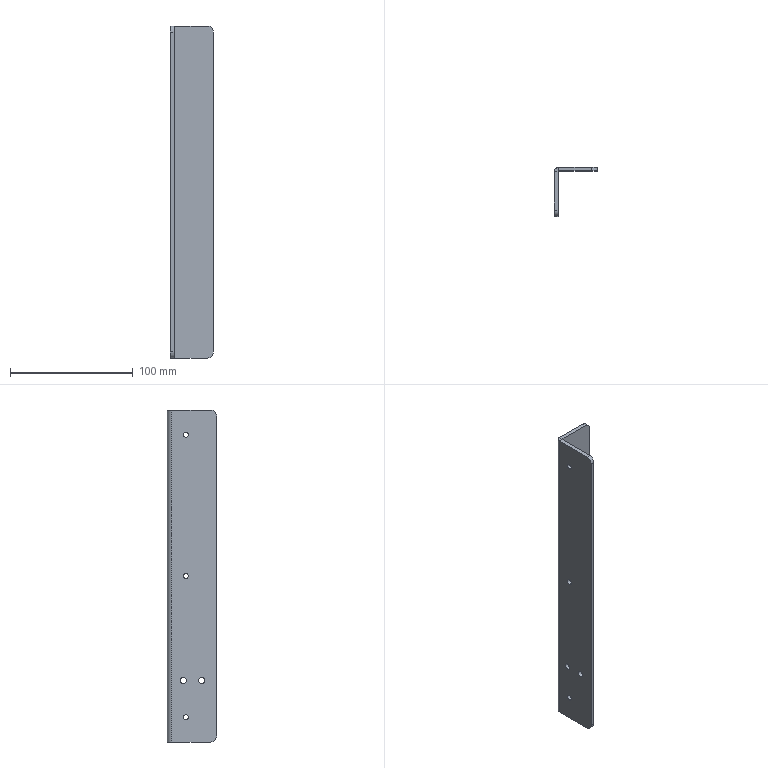Part | SolidWorks | features HoleWzd 2, Fillet 1, FlatPattern 1, SMBaseFlange 1, SheetMetal 1 | 1 solid | 28 faces | box 35 x 40 x 270 mm | volume 57353 mm3 | cylinder 16 | plane 12 | commonest cylinder face diameters 4.2 x6 5 x4 10 x4 0.8 x1 6.8 x1
STEP:
#1=CARTESIAN_POINT('',(-32.,-13.,-82.5));
#2=VERTEX_POINT('',#1);
#3=CARTESIAN_POINT('',(-32.,-13.,-87.5));
#4=VERTEX_POINT('',#3);
#5=CARTESIAN_POINT('',(-32.,-13.,-85.));
#6=DIRECTION('',(1.,0.,0.));
#7=DIRECTION('',(0.,1.,0.));
#8=AXIS2_PLACEMENT_3D('',#5,#6,#7);
#9=CIRCLE('',#8,2.5);
#10=EDGE_CURVE('',#2,#4,#9,.T.);
#11=ORIENTED_EDGE('',*,*,#10,.T.);
#12=CARTESIAN_POINT('',(-35.,-13.,-87.5));
#13=VERTEX_POINT('',#12);
#14=CARTESIAN_POINT('',(-35.,-13.,-87.5));
#15=DIRECTION('',(-1.,0.,0.));
#16=VECTOR('',#15,1000.);
#17=LINE('',#14,#16);
#18=EDGE_CURVE('',#4,#13,#17,.T.);
#19=ORIENTED_EDGE('',*,*,#18,.T.);
#20=CARTESIAN_POINT('',(-35.,-13.,-82.5));
#21=VERTEX_POINT('',#20);
#22=CARTESIAN_POINT('',(-35.,-13.,-85.));
#23=DIRECTION('',(-1.,0.,0.));
#24=DIRECTION('',(0.,0.,1.));
#25=AXIS2_PLACEMENT_3D('',#22,#23,#24);
#26=CIRCLE('',#25,2.5);
#27=EDGE_CURVE('',#13,#21,#26,.T.);
#28=ORIENTED_EDGE('',*,*,#27,.T.);
#29=CARTESIAN_POINT('',(-35.,-13.,-82.5));
#30=DIRECTION('',(-1.,0.,0.));
#31=VECTOR('',#30,1000.);
#32=LINE('',#29,#31);
#33=EDGE_CURVE('',#2,#21,#32,.T.);
#34=ORIENTED_EDGE('',*,*,#33,.F.);
#35=EDGE_LOOP('',(#11,#19,#28,#34));
#36=FACE_OUTER_BOUND('',#35,.T.);
#37=CARTESIAN_POINT('',(-35.,-13.,-85.));
#38=DIRECTION('',(-1.,0.,0.));
#39=DIRECTION('',(0.,0.,1.));
#40=AXIS2_PLACEMENT_3D('',#37,#38,#39);
#41=CYLINDRICAL_SURFACE('',#40,2.5);
#42=ADVANCED_FACE('',(#36),#41,.F.);
#43=CARTESIAN_POINT('',(-32.,-28.,-82.5));
#44=VERTEX_POINT('',#43);
#45=CARTESIAN_POINT('',(-32.,-28.,-87.5));
#46=VERTEX_POINT('',#45);
#47=CARTESIAN_POINT('',(-32.,-28.,-85.));
#48=DIRECTION('',(1.,0.,0.));
#49=DIRECTION('',(0.,1.,0.));
#50=AXIS2_PLACEMENT_3D('',#47,#48,#49);
#51=CIRCLE('',#50,2.5);
#52=EDGE_CURVE('',#44,#46,#51,.T.);
#53=ORIENTED_EDGE('',*,*,#52,.T.);
#54=CARTESIAN_POINT('',(-35.,-28.,-87.5));
#55=VERTEX_POINT('',#54);
#56=CARTESIAN_POINT('',(-35.,-28.,-87.5));
#57=DIRECTION('',(-1.,0.,0.));
#58=VECTOR('',#57,1000.);
#59=LINE('',#56,#58);
#60=EDGE_CURVE('',#46,#55,#59,.T.);
#61=ORIENTED_EDGE('',*,*,#60,.T.);
#62=CARTESIAN_POINT('',(-35.,-28.,-82.5));
#63=VERTEX_POINT('',#62);
#64=CARTESIAN_POINT('',(-35.,-28.,-85.));
#65=DIRECTION('',(-1.,0.,0.));
#66=DIRECTION('',(0.,0.,1.));
#67=AXIS2_PLACEMENT_3D('',#64,#65,#66);
#68=CIRCLE('',#67,2.5);
#69=EDGE_CURVE('',#55,#63,#68,.T.);
#70=ORIENTED_EDGE('',*,*,#69,.T.);
#71=CARTESIAN_POINT('',(-35.,-28.,-82.5));
#72=DIRECTION('',(-1.,0.,0.));
#73=VECTOR('',#72,1000.);
#74=LINE('',#71,#73);
#75=EDGE_CURVE('',#44,#63,#74,.T.);
#76=ORIENTED_EDGE('',*,*,#75,.F.);
#77=EDGE_LOOP('',(#53,#61,#70,#76));
#78=FACE_OUTER_BOUND('',#77,.T.);
#79=CARTESIAN_POINT('',(-35.,-28.,-85.));
#80=DIRECTION('',(-1.,0.,0.));
#81=DIRECTION('',(0.,0.,1.));
#82=AXIS2_PLACEMENT_3D('',#79,#80,#81);
#83=CYLINDRICAL_SURFACE('',#82,2.5);
#84=ADVANCED_FACE('',(#78),#83,.F.);
#85=CARTESIAN_POINT('',(-35.,-15.,117.1));
#86=VERTEX_POINT('',#85);
#87=CARTESIAN_POINT('',(-35.,-15.,112.9));
#88=VERTEX_POINT('',#87);
#89=CARTESIAN_POINT('',(-35.,-15.,115.));
#90=DIRECTION('',(1.,0.,0.));
#91=DIRECTION('',(0.,1.,0.));
#92=AXIS2_PLACEMENT_3D('',#89,#90,#91);
#93=CIRCLE('',#92,2.1);
#94=EDGE_CURVE('',#86,#88,#93,.T.);
#95=ORIENTED_EDGE('',*,*,#94,.F.);
#96=CARTESIAN_POINT('',(-32.,-15.,117.1));
#97=VERTEX_POINT('',#96);
#98=CARTESIAN_POINT('',(-32.,-15.,117.1));
#99=DIRECTION('',(1.,0.,0.));
#100=VECTOR('',#99,1000.);
#101=LINE('',#98,#100);
#102=EDGE_CURVE('',#86,#97,#101,.T.);
#103=ORIENTED_EDGE('',*,*,#102,.T.);
#104=CARTESIAN_POINT('',(-32.,-15.,112.9));
#105=VERTEX_POINT('',#104);
#106=CARTESIAN_POINT('',(-32.,-15.,115.));
#107=DIRECTION('',(1.,0.,0.));
#108=DIRECTION('',(0.,0.,-1.));
#109=AXIS2_PLACEMENT_3D('',#106,#107,#108);
#110=CIRCLE('',#109,2.1);
#111=EDGE_CURVE('',#97,#105,#110,.T.);
#112=ORIENTED_EDGE('',*,*,#111,.T.);
#113=CARTESIAN_POINT('',(-32.,-15.,112.9));
#114=DIRECTION('',(1.,0.,0.));
#115=VECTOR('',#114,1000.);
#116=LINE('',#113,#115);
#117=EDGE_CURVE('',#88,#105,#116,.T.);
#118=ORIENTED_EDGE('',*,*,#117,.F.);
#119=EDGE_LOOP('',(#95,#103,#112,#118));
#120=FACE_OUTER_BOUND('',#119,.T.);
#121=CARTESIAN_POINT('',(-32.,-15.,115.));
#122=DIRECTION('',(1.,0.,0.));
#123=DIRECTION('',(0.,0.,-1.));
#124=AXIS2_PLACEMENT_3D('',#121,#122,#123);
#125=CYLINDRICAL_SURFACE('',#124,2.1);
#126=ADVANCED_FACE('',(#120),#125,.F.);
#127=CARTESIAN_POINT('',(-35.,-15.,-112.9));
#128=VERTEX_POINT('',#127);
#129=CARTESIAN_POINT('',(-35.,-15.,-117.1));
#130=VERTEX_POINT('',#129);
#131=CARTESIAN_POINT('',(-35.,-15.,-115.));
#132=DIRECTION('',(1.,0.,0.));
#133=DIRECTION('',(0.,1.,0.));
#134=AXIS2_PLACEMENT_3D('',#131,#132,#133);
#135=CIRCLE('',#134,2.1);
#136=EDGE_CURVE('',#128,#130,#135,.T.);
#137=ORIENTED_EDGE('',*,*,#136,.F.);
#138=CARTESIAN_POINT('',(-32.,-15.,-112.9));
#139=VERTEX_POINT('',#138);
#140=CARTESIAN_POINT('',(-32.,-15.,-112.9));
#141=DIRECTION('',(1.,0.,0.));
#142=VECTOR('',#141,1000.);
#143=LINE('',#140,#142);
#144=EDGE_CURVE('',#128,#139,#143,.T.);
#145=ORIENTED_EDGE('',*,*,#144,.T.);
#146=CARTESIAN_POINT('',(-32.,-15.,-117.1));
#147=VERTEX_POINT('',#146);
#148=CARTESIAN_POINT('',(-32.,-15.,-115.));
#149=DIRECTION('',(1.,0.,0.));
#150=DIRECTION('',(0.,0.,-1.));
#151=AXIS2_PLACEMENT_3D('',#148,#149,#150);
#152=CIRCLE('',#151,2.1);
#153=EDGE_CURVE('',#139,#147,#152,.T.);
#154=ORIENTED_EDGE('',*,*,#153,.T.);
#155=CARTESIAN_POINT('',(-32.,-15.,-117.1));
#156=DIRECTION('',(1.,0.,0.));
#157=VECTOR('',#156,1000.);
#158=LINE('',#155,#157);
#159=EDGE_CURVE('',#130,#147,#158,.T.);
#160=ORIENTED_EDGE('',*,*,#159,.F.);
#161=EDGE_LOOP('',(#137,#145,#154,#160));
#162=FACE_OUTER_BOUND('',#161,.T.);
#163=CARTESIAN_POINT('',(-32.,-15.,-115.));
#164=DIRECTION('',(1.,0.,0.));
#165=DIRECTION('',(0.,0.,-1.));
#166=AXIS2_PLACEMENT_3D('',#163,#164,#165);
#167=CYLINDRICAL_SURFACE('',#166,2.1);
#168=ADVANCED_FACE('',(#162),#167,.F.);
#169=CARTESIAN_POINT('',(-35.,-15.,2.1));
#170=VERTEX_POINT('',#169);
#171=CARTESIAN_POINT('',(-35.,-15.,-2.1));
#172=VERTEX_POINT('',#171);
#173=CARTESIAN_POINT('',(-35.,-15.,0.));
#174=DIRECTION('',(1.,0.,0.));
#175=DIRECTION('',(0.,1.,0.));
#176=AXIS2_PLACEMENT_3D('',#173,#174,#175);
#177=CIRCLE('',#176,2.1);
#178=EDGE_CURVE('',#170,#172,#177,.T.);
#179=ORIENTED_EDGE('',*,*,#178,.F.);
#180=CARTESIAN_POINT('',(-32.,-15.,2.1));
#181=VERTEX_POINT('',#180);
#182=CARTESIAN_POINT('',(-32.,-15.,2.1));
#183=DIRECTION('',(1.,0.,0.));
#184=VECTOR('',#183,1000.);
#185=LINE('',#182,#184);
#186=EDGE_CURVE('',#170,#181,#185,.T.);
#187=ORIENTED_EDGE('',*,*,#186,.T.);
#188=CARTESIAN_POINT('',(-32.,-15.,-2.1));
#189=VERTEX_POINT('',#188);
#190=CARTESIAN_POINT('',(-32.,-15.,0.));
#191=DIRECTION('',(1.,0.,0.));
#192=DIRECTION('',(0.,0.,-1.));
#193=AXIS2_PLACEMENT_3D('',#190,#191,#192);
#194=CIRCLE('',#193,2.1);
#195=EDGE_CURVE('',#181,#189,#194,.T.);
#196=ORIENTED_EDGE('',*,*,#195,.T.);
#197=CARTESIAN_POINT('',(-32.,-15.,-2.1));
#198=DIRECTION('',(1.,0.,0.));
#199=VECTOR('',#198,1000.);
#200=LINE('',#197,#199);
#201=EDGE_CURVE('',#172,#189,#200,.T.);
#202=ORIENTED_EDGE('',*,*,#201,.F.);
#203=EDGE_LOOP('',(#179,#187,#196,#202));
#204=FACE_OUTER_BOUND('',#203,.T.);
#205=CARTESIAN_POINT('',(-32.,-15.,0.));
#206=DIRECTION('',(1.,0.,0.));
#207=DIRECTION('',(0.,0.,-1.));
#208=AXIS2_PLACEMENT_3D('',#205,#206,#207);
#209=CYLINDRICAL_SURFACE('',#208,2.1);
#210=ADVANCED_FACE('',(#204),#209,.F.);
#211=CARTESIAN_POINT('',(-31.6,0.,135.));
#212=VERTEX_POINT('',#211);
#213=CARTESIAN_POINT('',(-31.6,-3.,135.));
#214=VERTEX_POINT('',#213);
#215=CARTESIAN_POINT('',(-31.6,0.,135.));
#216=DIRECTION('',(0.,-1.,0.));
#217=VECTOR('',#216,1000.);
#218=LINE('',#215,#217);
#219=EDGE_CURVE('',#212,#214,#218,.T.);
#220=ORIENTED_EDGE('',*,*,#219,.F.);
#221=CARTESIAN_POINT('',(-35.,-3.4,135.));
#222=VERTEX_POINT('',#221);
#223=CARTESIAN_POINT('',(-31.6,-3.4,135.));
#224=DIRECTION('',(0.,0.,1.));
#225=DIRECTION('',(-1.,0.,0.));
#226=AXIS2_PLACEMENT_3D('',#223,#224,#225);
#227=CIRCLE('',#226,3.4);
#228=EDGE_CURVE('',#212,#222,#227,.T.);
#229=ORIENTED_EDGE('',*,*,#228,.T.);
#230=CARTESIAN_POINT('',(-32.,-3.4,135.));
#231=VERTEX_POINT('',#230);
#232=CARTESIAN_POINT('',(-32.,-3.4,135.));
#233=DIRECTION('',(-1.,0.,0.));
#234=VECTOR('',#233,1000.);
#235=LINE('',#232,#234);
#236=EDGE_CURVE('',#231,#222,#235,.T.);
#237=ORIENTED_EDGE('',*,*,#236,.F.);
#238=CARTESIAN_POINT('',(-31.6,-3.4,135.));
#239=DIRECTION('',(0.,0.,1.));
#240=DIRECTION('',(1.,0.,0.));
#241=AXIS2_PLACEMENT_3D('',#238,#239,#240);
#242=CIRCLE('',#241,0.4);
#243=EDGE_CURVE('',#214,#231,#242,.T.);
#244=ORIENTED_EDGE('',*,*,#243,.F.);
#245=EDGE_LOOP('',(#220,#229,#237,#244));
#246=FACE_OUTER_BOUND('',#245,.T.);
#247=CARTESIAN_POINT('',(-31.6,0.,135.));
#248=DIRECTION('',(0.,0.,1.));
#249=DIRECTION('',(1.,0.,0.));
#250=AXIS2_PLACEMENT_3D('',#247,#248,#249);
#251=PLANE('',#250);
#252=ADVANCED_FACE('',(#246),#251,.T.);
#253=CARTESIAN_POINT('',(-5.,-3.,135.));
#254=VERTEX_POINT('',#253);
#255=CARTESIAN_POINT('',(0.,-3.,135.));
#256=DIRECTION('',(-1.,0.,0.));
#257=VECTOR('',#256,1000.);
#258=LINE('',#255,#257);
#259=EDGE_CURVE('',#254,#214,#258,.T.);
#260=ORIENTED_EDGE('',*,*,#259,.F.);
#261=CARTESIAN_POINT('',(-5.,0.,135.));
#262=VERTEX_POINT('',#261);
#263=CARTESIAN_POINT('',(-5.,-3.4,135.));
#264=DIRECTION('',(0.,1.,0.));
#265=VECTOR('',#264,1000.);
#266=LINE('',#263,#265);
#267=EDGE_CURVE('',#254,#262,#266,.T.);
#268=ORIENTED_EDGE('',*,*,#267,.T.);
#269=CARTESIAN_POINT('',(0.,0.,135.));
#270=DIRECTION('',(-1.,0.,0.));
#271=VECTOR('',#270,1000.);
#272=LINE('',#269,#271);
#273=EDGE_CURVE('',#262,#212,#272,.T.);
#274=ORIENTED_EDGE('',*,*,#273,.T.);
#275=ORIENTED_EDGE('',*,*,#219,.T.);
#276=EDGE_LOOP('',(#260,#268,#274,#275));
#277=FACE_OUTER_BOUND('',#276,.T.);
#278=CARTESIAN_POINT('',(-32.,-3.4,135.));
#279=DIRECTION('',(0.,0.,1.));
#280=DIRECTION('',(1.,0.,0.));
#281=AXIS2_PLACEMENT_3D('',#278,#279,#280);
#282=PLANE('',#281);
#283=ADVANCED_FACE('',(#277),#282,.T.);
#284=CARTESIAN_POINT('',(-35.,-3.4,-135.));
#285=VERTEX_POINT('',#284);
#286=CARTESIAN_POINT('',(-32.,-3.4,-135.));
#287=VERTEX_POINT('',#286);
#288=CARTESIAN_POINT('',(-35.,-3.4,-135.));
#289=DIRECTION('',(1.,0.,0.));
#290=VECTOR('',#289,1000.);
#291=LINE('',#288,#290);
#292=EDGE_CURVE('',#285,#287,#291,.T.);
#293=ORIENTED_EDGE('',*,*,#292,.F.);
#294=CARTESIAN_POINT('',(-31.6,0.,-135.));
#295=VERTEX_POINT('',#294);
#296=CARTESIAN_POINT('',(-31.6,-3.4,-135.));
#297=DIRECTION('',(0.,0.,1.));
#298=DIRECTION('',(-1.,0.,0.));
#299=AXIS2_PLACEMENT_3D('',#296,#297,#298);
#300=CIRCLE('',#299,3.4);
#301=EDGE_CURVE('',#295,#285,#300,.T.);
#302=ORIENTED_EDGE('',*,*,#301,.F.);
#303=CARTESIAN_POINT('',(-31.6,-3.,-135.));
#304=VERTEX_POINT('',#303);
#305=CARTESIAN_POINT('',(-31.6,-3.,-135.));
#306=DIRECTION('',(0.,1.,0.));
#307=VECTOR('',#306,1000.);
#308=LINE('',#305,#307);
#309=EDGE_CURVE('',#304,#295,#308,.T.);
#310=ORIENTED_EDGE('',*,*,#309,.F.);
#311=CARTESIAN_POINT('',(-31.6,-3.4,-135.));
#312=DIRECTION('',(0.,0.,1.));
#313=DIRECTION('',(1.,0.,0.));
#314=AXIS2_PLACEMENT_3D('',#311,#312,#313);
#315=CIRCLE('',#314,0.4);
#316=EDGE_CURVE('',#304,#287,#315,.T.);
#317=ORIENTED_EDGE('',*,*,#316,.T.);
#318=EDGE_LOOP('',(#293,#302,#310,#317));
#319=FACE_OUTER_BOUND('',#318,.T.);
#320=CARTESIAN_POINT('',(-35.,-3.4,-135.));
#321=DIRECTION('',(0.,0.,-1.));
#322=DIRECTION('',(-1.,0.,0.));
#323=AXIS2_PLACEMENT_3D('',#320,#321,#322);
#324=PLANE('',#323);
#325=ADVANCED_FACE('',(#319),#324,.T.);
#326=CARTESIAN_POINT('',(-32.,-35.,-135.));
#327=VERTEX_POINT('',#326);
#328=CARTESIAN_POINT('',(-32.,0.,-135.));
#329=DIRECTION('',(0.,-1.,0.));
#330=VECTOR('',#329,1000.);
#331=LINE('',#328,#330);
#332=EDGE_CURVE('',#287,#327,#331,.T.);
#333=ORIENTED_EDGE('',*,*,#332,.T.);
#334=CARTESIAN_POINT('',(-35.,-35.,-135.));
#335=VERTEX_POINT('',#334);
#336=CARTESIAN_POINT('',(-31.6,-35.,-135.));
#337=DIRECTION('',(-1.,0.,0.));
#338=VECTOR('',#337,1000.);
#339=LINE('',#336,#338);
#340=EDGE_CURVE('',#327,#335,#339,.T.);
#341=ORIENTED_EDGE('',*,*,#340,.T.);
#342=CARTESIAN_POINT('',(-35.,0.,-135.));
#343=DIRECTION('',(0.,-1.,0.));
#344=VECTOR('',#343,1000.);
#345=LINE('',#342,#344);
#346=EDGE_CURVE('',#285,#335,#345,.T.);
#347=ORIENTED_EDGE('',*,*,#346,.F.);
#348=ORIENTED_EDGE('',*,*,#292,.T.);
#349=EDGE_LOOP('',(#333,#341,#347,#348));
#350=FACE_OUTER_BOUND('',#349,.T.);
#351=CARTESIAN_POINT('',(-31.6,-3.,-135.));
#352=DIRECTION('',(0.,0.,-1.));
#353=DIRECTION('',(-1.,0.,0.));
#354=AXIS2_PLACEMENT_3D('',#351,#352,#353);
#355=PLANE('',#354);
#356=ADVANCED_FACE('',(#350),#355,.T.);
#357=CARTESIAN_POINT('',(-35.,-13.,-85.));
#358=DIRECTION('',(-1.,0.,0.));
#359=DIRECTION('',(0.,0.,1.));
#360=AXIS2_PLACEMENT_3D('',#357,#358,#359);
#361=CIRCLE('',#360,2.5);
#362=EDGE_CURVE('',#21,#13,#361,.T.);
#363=ORIENTED_EDGE('',*,*,#362,.F.);
#364=ORIENTED_EDGE('',*,*,#27,.F.);
#365=EDGE_LOOP('',(#363,#364));
#366=FACE_BOUND('',#365,.T.);
#367=CARTESIAN_POINT('',(-35.,-28.,-85.));
#368=DIRECTION('',(-1.,0.,0.));
#369=DIRECTION('',(0.,0.,1.));
#370=AXIS2_PLACEMENT_3D('',#367,#368,#369);
#371=CIRCLE('',#370,2.5);
#372=EDGE_CURVE('',#63,#55,#371,.T.);
#373=ORIENTED_EDGE('',*,*,#372,.F.);
#374=ORIENTED_EDGE('',*,*,#69,.F.);
#375=EDGE_LOOP('',(#373,#374));
#376=FACE_BOUND('',#375,.T.);
#377=CARTESIAN_POINT('',(-35.,-15.,115.));
#378=DIRECTION('',(1.,0.,0.));
#379=DIRECTION('',(0.,1.,0.));
#380=AXIS2_PLACEMENT_3D('',#377,#378,#379);
#381=CIRCLE('',#380,2.1);
#382=EDGE_CURVE('',#88,#86,#381,.T.);
#383=ORIENTED_EDGE('',*,*,#382,.T.);
#384=ORIENTED_EDGE('',*,*,#94,.T.);
#385=EDGE_LOOP('',(#383,#384));
#386=FACE_BOUND('',#385,.T.);
#387=CARTESIAN_POINT('',(-35.,-15.,-115.));
#388=DIRECTION('',(1.,0.,0.));
#389=DIRECTION('',(0.,1.,0.));
#390=AXIS2_PLACEMENT_3D('',#387,#388,#389);
#391=CIRCLE('',#390,2.1);
#392=EDGE_CURVE('',#130,#128,#391,.T.);
#393=ORIENTED_EDGE('',*,*,#392,.T.);
#394=ORIENTED_EDGE('',*,*,#136,.T.);
#395=EDGE_LOOP('',(#393,#394));
#396=FACE_BOUND('',#395,.T.);
#397=CARTESIAN_POINT('',(-35.,-15.,0.));
#398=DIRECTION('',(1.,0.,0.));
#399=DIRECTION('',(0.,1.,0.));
#400=AXIS2_PLACEMENT_3D('',#397,#398,#399);
#401=CIRCLE('',#400,2.1);
#402=EDGE_CURVE('',#172,#170,#401,.T.);
#403=ORIENTED_EDGE('',*,*,#402,.T.);
#404=ORIENTED_EDGE('',*,*,#178,.T.);
#405=EDGE_LOOP('',(#403,#404));
#406=FACE_BOUND('',#405,.T.);
#407=ORIENTED_EDGE('',*,*,#346,.T.);
#408=CARTESIAN_POINT('',(-35.,-40.,-130.));
#409=VERTEX_POINT('',#408);
#410=CARTESIAN_POINT('',(-35.,-35.,-130.));
#411=DIRECTION('',(-1.,0.,0.));
#412=DIRECTION('',(0.,1.,0.));
#413=AXIS2_PLACEMENT_3D('',#410,#411,#412);
#414=CIRCLE('',#413,5.);
#415=EDGE_CURVE('',#335,#409,#414,.T.);
#416=ORIENTED_EDGE('',*,*,#415,.T.);
#417=CARTESIAN_POINT('',(-35.,-40.,130.));
#418=VERTEX_POINT('',#417);
#419=CARTESIAN_POINT('',(-35.,-40.,135.));
#420=DIRECTION('',(0.,0.,-1.));
#421=VECTOR('',#420,1000.);
#422=LINE('',#419,#421);
#423=EDGE_CURVE('',#418,#409,#422,.T.);
#424=ORIENTED_EDGE('',*,*,#423,.F.);
#425=CARTESIAN_POINT('',(-35.,-35.,135.));
#426=VERTEX_POINT('',#425);
#427=CARTESIAN_POINT('',(-35.,-35.,130.));
#428=DIRECTION('',(-1.,0.,0.));
#429=DIRECTION('',(0.,1.,0.));
#430=AXIS2_PLACEMENT_3D('',#427,#428,#429);
#431=CIRCLE('',#430,5.);
#432=EDGE_CURVE('',#418,#426,#431,.T.);
#433=ORIENTED_EDGE('',*,*,#432,.T.);
#434=CARTESIAN_POINT('',(-35.,0.,135.));
#435=DIRECTION('',(0.,-1.,0.));
#436=VECTOR('',#435,1000.);
#437=LINE('',#434,#436);
#438=EDGE_CURVE('',#222,#426,#437,.T.);
#439=ORIENTED_EDGE('',*,*,#438,.F.);
#440=CARTESIAN_POINT('',(-35.,-3.4,135.));
#441=DIRECTION('',(0.,0.,-1.));
#442=VECTOR('',#441,1000.);
#443=LINE('',#440,#442);
#444=EDGE_CURVE('',#222,#285,#443,.T.);
#445=ORIENTED_EDGE('',*,*,#444,.T.);
#446=EDGE_LOOP('',(#407,#416,#424,#433,#439,#445));
#447=FACE_OUTER_BOUND('',#446,.T.);
#448=CARTESIAN_POINT('',(-35.,0.,135.));
#449=DIRECTION('',(1.,0.,0.));
#450=DIRECTION('',(0.,1.,0.));
#451=AXIS2_PLACEMENT_3D('',#448,#449,#450);
#452=PLANE('',#451);
#453=ADVANCED_FACE('',(#366,#376,#386,#396,#406,#447),#452,.F.);
#454=ORIENTED_EDGE('',*,*,#423,.T.);
#455=CARTESIAN_POINT('',(-32.,-40.,-130.));
#456=VERTEX_POINT('',#455);
#457=CARTESIAN_POINT('',(-32.,-40.,-130.));
#458=DIRECTION('',(1.,0.,0.));
#459=VECTOR('',#458,1000.);
#460=LINE('',#457,#459);
#461=EDGE_CURVE('',#409,#456,#460,.T.);
#462=ORIENTED_EDGE('',*,*,#461,.T.);
#463=CARTESIAN_POINT('',(-32.,-40.,130.));
#464=VERTEX_POINT('',#463);
#465=CARTESIAN_POINT('',(-32.,-40.,135.));
#466=DIRECTION('',(0.,0.,-1.));
#467=VECTOR('',#466,1000.);
#468=LINE('',#465,#467);
#469=EDGE_CURVE('',#464,#456,#468,.T.);
#470=ORIENTED_EDGE('',*,*,#469,.F.);
#471=CARTESIAN_POINT('',(-32.,-40.,130.));
#472=DIRECTION('',(-1.,0.,0.));
#473=VECTOR('',#472,1000.);
#474=LINE('',#471,#473);
#475=EDGE_CURVE('',#464,#418,#474,.T.);
#476=ORIENTED_EDGE('',*,*,#475,.T.);
#477=EDGE_LOOP('',(#454,#462,#470,#476));
#478=FACE_OUTER_BOUND('',#477,.T.);
#479=CARTESIAN_POINT('',(-32.,-40.,135.));
#480=DIRECTION('',(0.,-1.,0.));
#481=DIRECTION('',(0.,0.,-1.));
#482=AXIS2_PLACEMENT_3D('',#479,#480,#481);
#483=PLANE('',#482);
#484=ADVANCED_FACE('',(#478),#483,.T.);
#485=ORIENTED_EDGE('',*,*,#10,.F.);
#486=CARTESIAN_POINT('',(-32.,-13.,-85.));
#487=DIRECTION('',(1.,0.,0.));
#488=DIRECTION('',(0.,1.,0.));
#489=AXIS2_PLACEMENT_3D('',#486,#487,#488);
#490=CIRCLE('',#489,2.5);
#491=EDGE_CURVE('',#4,#2,#490,.T.);
#492=ORIENTED_EDGE('',*,*,#491,.F.);
#493=EDGE_LOOP('',(#485,#492));
#494=FACE_BOUND('',#493,.T.);
#495=ORIENTED_EDGE('',*,*,#52,.F.);
#496=CARTESIAN_POINT('',(-32.,-28.,-85.));
#497=DIRECTION('',(1.,0.,0.));
#498=DIRECTION('',(0.,1.,0.));
#499=AXIS2_PLACEMENT_3D('',#496,#497,#498);
#500=CIRCLE('',#499,2.5);
#501=EDGE_CURVE('',#46,#44,#500,.T.);
#502=ORIENTED_EDGE('',*,*,#501,.F.);
#503=EDGE_LOOP('',(#495,#502));
#504=FACE_BOUND('',#503,.T.);
#505=CARTESIAN_POINT('',(-32.,-15.,115.));
#506=DIRECTION('',(1.,0.,0.));
#507=DIRECTION('',(0.,0.,-1.));
#508=AXIS2_PLACEMENT_3D('',#505,#506,#507);
#509=CIRCLE('',#508,2.1);
#510=EDGE_CURVE('',#105,#97,#509,.T.);
#511=ORIENTED_EDGE('',*,*,#510,.F.);
#512=ORIENTED_EDGE('',*,*,#111,.F.);
#513=EDGE_LOOP('',(#511,#512));
#514=FACE_BOUND('',#513,.T.);
#515=CARTESIAN_POINT('',(-32.,-15.,-115.));
#516=DIRECTION('',(1.,0.,0.));
#517=DIRECTION('',(0.,0.,-1.));
#518=AXIS2_PLACEMENT_3D('',#515,#516,#517);
#519=CIRCLE('',#518,2.1);
#520=EDGE_CURVE('',#147,#139,#519,.T.);
#521=ORIENTED_EDGE('',*,*,#520,.F.);
#522=ORIENTED_EDGE('',*,*,#153,.F.);
#523=EDGE_LOOP('',(#521,#522));
#524=FACE_BOUND('',#523,.T.);
#525=CARTESIAN_POINT('',(-32.,-15.,0.));
#526=DIRECTION('',(1.,0.,0.));
#527=DIRECTION('',(0.,0.,-1.));
#528=AXIS2_PLACEMENT_3D('',#525,#526,#527);
#529=CIRCLE('',#528,2.1);
#530=EDGE_CURVE('',#189,#181,#529,.T.);
#531=ORIENTED_EDGE('',*,*,#530,.F.);
#532=ORIENTED_EDGE('',*,*,#195,.F.);
#533=EDGE_LOOP('',(#531,#532));
#534=FACE_BOUND('',#533,.T.);
#535=ORIENTED_EDGE('',*,*,#469,.T.);
#536=CARTESIAN_POINT('',(-32.,-35.,-130.));
#537=DIRECTION('',(1.,0.,0.));
#538=DIRECTION('',(0.,1.,0.));
#539=AXIS2_PLACEMENT_3D('',#536,#537,#538);
#540=CIRCLE('',#539,5.);
#541=EDGE_CURVE('',#456,#327,#540,.T.);
#542=ORIENTED_EDGE('',*,*,#541,.T.);
#543=ORIENTED_EDGE('',*,*,#332,.F.);
#544=CARTESIAN_POINT('',(-32.,-3.4,135.));
#545=DIRECTION('',(0.,0.,-1.));
#546=VECTOR('',#545,1000.);
#547=LINE('',#544,#546);
#548=EDGE_CURVE('',#231,#287,#547,.T.);
#549=ORIENTED_EDGE('',*,*,#548,.F.);
#550=CARTESIAN_POINT('',(-32.,-35.,135.));
#551=VERTEX_POINT('',#550);
#552=CARTESIAN_POINT('',(-32.,0.,135.));
#553=DIRECTION('',(0.,-1.,0.));
#554=VECTOR('',#553,1000.);
#555=LINE('',#552,#554);
#556=EDGE_CURVE('',#231,#551,#555,.T.);
#557=ORIENTED_EDGE('',*,*,#556,.T.);
#558=CARTESIAN_POINT('',(-32.,-35.,130.));
#559=DIRECTION('',(1.,0.,0.));
#560=DIRECTION('',(0.,1.,0.));
#561=AXIS2_PLACEMENT_3D('',#558,#559,#560);
#562=CIRCLE('',#561,5.);
#563=EDGE_CURVE('',#551,#464,#562,.T.);
#564=ORIENTED_EDGE('',*,*,#563,.T.);
#565=EDGE_LOOP('',(#535,#542,#543,#549,#557,#564));
#566=FACE_OUTER_BOUND('',#565,.T.);
#567=CARTESIAN_POINT('',(-32.,0.,135.));
#568=DIRECTION('',(1.,0.,0.));
#569=DIRECTION('',(0.,1.,0.));
#570=AXIS2_PLACEMENT_3D('',#567,#568,#569);
#571=PLANE('',#570);
#572=ADVANCED_FACE('',(#494,#504,#514,#524,#534,#566),#571,.T.);
#573=ORIENTED_EDGE('',*,*,#316,.F.);
#574=CARTESIAN_POINT('',(-31.6,-3.,135.));
#575=DIRECTION('',(0.,0.,-1.));
#576=VECTOR('',#575,1000.);
#577=LINE('',#574,#576);
#578=EDGE_CURVE('',#214,#304,#577,.T.);
#579=ORIENTED_EDGE('',*,*,#578,.F.);
#580=ORIENTED_EDGE('',*,*,#243,.T.);
#581=ORIENTED_EDGE('',*,*,#548,.T.);
#582=EDGE_LOOP('',(#573,#579,#580,#581));
#583=FACE_OUTER_BOUND('',#582,.T.);
#584=CARTESIAN_POINT('',(-31.6,-3.4,135.));
#585=DIRECTION('',(0.,0.,-1.));
#586=DIRECTION('',(-1.,0.,0.));
#587=AXIS2_PLACEMENT_3D('',#584,#585,#586);
#588=CYLINDRICAL_SURFACE('',#587,0.4);
#589=ADVANCED_FACE('',(#583),#588,.F.);
#590=CARTESIAN_POINT('',(-5.,-3.,-135.));
#591=VERTEX_POINT('',#590);
#592=CARTESIAN_POINT('',(0.,-3.,-135.));
#593=DIRECTION('',(-1.,0.,0.));
#594=VECTOR('',#593,1000.);
#595=LINE('',#592,#594);
#596=EDGE_CURVE('',#591,#304,#595,.T.);
#597=ORIENTED_EDGE('',*,*,#596,.F.);
#598=CARTESIAN_POINT('',(0.,-3.,-130.));
#599=VERTEX_POINT('',#598);
#600=CARTESIAN_POINT('',(-5.,-3.,-130.));
#601=DIRECTION('',(0.,-1.,0.));
#602=DIRECTION('',(0.,0.,-1.));
#603=AXIS2_PLACEMENT_3D('',#600,#601,#602);
#604=CIRCLE('',#603,5.);
#605=EDGE_CURVE('',#591,#599,#604,.T.);
#606=ORIENTED_EDGE('',*,*,#605,.T.);
#607=CARTESIAN_POINT('',(0.,-3.,130.));
#608=VERTEX_POINT('',#607);
#609=CARTESIAN_POINT('',(0.,-3.,135.));
#610=DIRECTION('',(0.,0.,-1.));
#611=VECTOR('',#610,1000.);
#612=LINE('',#609,#611);
#613=EDGE_CURVE('',#608,#599,#612,.T.);
#614=ORIENTED_EDGE('',*,*,#613,.F.);
#615=CARTESIAN_POINT('',(-5.,-3.,130.));
#616=DIRECTION('',(0.,-1.,0.));
#617=DIRECTION('',(0.,0.,-1.));
#618=AXIS2_PLACEMENT_3D('',#615,#616,#617);
#619=CIRCLE('',#618,5.);
#620=EDGE_CURVE('',#608,#254,#619,.T.);
#621=ORIENTED_EDGE('',*,*,#620,.T.);
#622=ORIENTED_EDGE('',*,*,#259,.T.);
#623=ORIENTED_EDGE('',*,*,#578,.T.);
#624=EDGE_LOOP('',(#597,#606,#614,#621,#622,#623));
#625=FACE_OUTER_BOUND('',#624,.T.);
#626=CARTESIAN_POINT('',(0.,-3.,135.));
#627=DIRECTION('',(0.,-1.,0.));
#628=DIRECTION('',(0.,0.,-1.));
#629=AXIS2_PLACEMENT_3D('',#626,#627,#628);
#630=PLANE('',#629);
#631=ADVANCED_FACE('',(#625),#630,.T.);
#632=ORIENTED_EDGE('',*,*,#613,.T.);
#633=CARTESIAN_POINT('',(0.,0.,-130.));
#634=VERTEX_POINT('',#633);
#635=CARTESIAN_POINT('',(0.,0.,-130.));
#636=DIRECTION('',(0.,1.,0.));
#637=VECTOR('',#636,1000.);
#638=LINE('',#635,#637);
#639=EDGE_CURVE('',#599,#634,#638,.T.);
#640=ORIENTED_EDGE('',*,*,#639,.T.);
#641=CARTESIAN_POINT('',(0.,0.,130.));
#642=VERTEX_POINT('',#641);
#643=CARTESIAN_POINT('',(0.,0.,135.));
#644=DIRECTION('',(0.,0.,-1.));
#645=VECTOR('',#644,1000.);
#646=LINE('',#643,#645);
#647=EDGE_CURVE('',#642,#634,#646,.T.);
#648=ORIENTED_EDGE('',*,*,#647,.F.);
#649=CARTESIAN_POINT('',(0.,0.,130.));
#650=DIRECTION('',(0.,-1.,0.));
#651=VECTOR('',#650,1000.);
#652=LINE('',#649,#651);
#653=EDGE_CURVE('',#642,#608,#652,.T.);
#654=ORIENTED_EDGE('',*,*,#653,.T.);
#655=EDGE_LOOP('',(#632,#640,#648,#654));
#656=FACE_OUTER_BOUND('',#655,.T.);
#657=CARTESIAN_POINT('',(0.,0.,135.));
#658=DIRECTION('',(1.,0.,0.));
#659=DIRECTION('',(0.,0.,-1.));
#660=AXIS2_PLACEMENT_3D('',#657,#658,#659);
#661=PLANE('',#660);
#662=ADVANCED_FACE('',(#656),#661,.T.);
#663=ORIENTED_EDGE('',*,*,#647,.T.);
#664=CARTESIAN_POINT('',(-5.,0.,-135.));
#665=VERTEX_POINT('',#664);
#666=CARTESIAN_POINT('',(-5.,0.,-130.));
#667=DIRECTION('',(0.,1.,0.));
#668=DIRECTION('',(0.,0.,-1.));
#669=AXIS2_PLACEMENT_3D('',#666,#667,#668);
#670=CIRCLE('',#669,5.);
#671=EDGE_CURVE('',#634,#665,#670,.T.);
#672=ORIENTED_EDGE('',*,*,#671,.T.);
#673=CARTESIAN_POINT('',(0.,0.,-135.));
#674=DIRECTION('',(-1.,0.,0.));
#675=VECTOR('',#674,1000.);
#676=LINE('',#673,#675);
#677=EDGE_CURVE('',#665,#295,#676,.T.);
#678=ORIENTED_EDGE('',*,*,#677,.T.);
#679=CARTESIAN_POINT('',(-31.6,0.,135.));
#680=DIRECTION('',(0.,0.,-1.));
#681=VECTOR('',#680,1000.);
#682=LINE('',#679,#681);
#683=EDGE_CURVE('',#212,#295,#682,.T.);
#684=ORIENTED_EDGE('',*,*,#683,.F.);
#685=ORIENTED_EDGE('',*,*,#273,.F.);
#686=CARTESIAN_POINT('',(-5.,0.,130.));
#687=DIRECTION('',(0.,1.,0.));
#688=DIRECTION('',(0.,0.,-1.));
#689=AXIS2_PLACEMENT_3D('',#686,#687,#688);
#690=CIRCLE('',#689,5.);
#691=EDGE_CURVE('',#262,#642,#690,.T.);
#692=ORIENTED_EDGE('',*,*,#691,.T.);
#693=EDGE_LOOP('',(#663,#672,#678,#684,#685,#692));
#694=FACE_OUTER_BOUND('',#693,.T.);
#695=CARTESIAN_POINT('',(0.,0.,135.));
#696=DIRECTION('',(0.,-1.,0.));
#697=DIRECTION('',(0.,0.,-1.));
#698=AXIS2_PLACEMENT_3D('',#695,#696,#697);
#699=PLANE('',#698);
#700=ADVANCED_FACE('',(#694),#699,.F.);
#701=ORIENTED_EDGE('',*,*,#301,.T.);
#702=ORIENTED_EDGE('',*,*,#444,.F.);
#703=ORIENTED_EDGE('',*,*,#228,.F.);
#704=ORIENTED_EDGE('',*,*,#683,.T.);
#705=EDGE_LOOP('',(#701,#702,#703,#704));
#706=FACE_OUTER_BOUND('',#705,.T.);
#707=CARTESIAN_POINT('',(-31.6,-3.4,135.));
#708=DIRECTION('',(0.,0.,-1.));
#709=DIRECTION('',(-1.,0.,0.));
#710=AXIS2_PLACEMENT_3D('',#707,#708,#709);
#711=CYLINDRICAL_SURFACE('',#710,3.4);
#712=ADVANCED_FACE('',(#706),#711,.T.);
#713=ORIENTED_EDGE('',*,*,#438,.T.);
#714=CARTESIAN_POINT('',(-31.6,-35.,135.));
#715=DIRECTION('',(1.,0.,0.));
#716=VECTOR('',#715,1000.);
#717=LINE('',#714,#716);
#718=EDGE_CURVE('',#426,#551,#717,.T.);
#719=ORIENTED_EDGE('',*,*,#718,.T.);
#720=ORIENTED_EDGE('',*,*,#556,.F.);
#721=ORIENTED_EDGE('',*,*,#236,.T.);
#722=EDGE_LOOP('',(#713,#719,#720,#721));
#723=FACE_OUTER_BOUND('',#722,.T.);
#724=CARTESIAN_POINT('',(-31.6,-3.4,135.));
#725=DIRECTION('',(0.,0.,1.));
#726=DIRECTION('',(1.,0.,0.));
#727=AXIS2_PLACEMENT_3D('',#724,#725,#726);
#728=PLANE('',#727);
#729=ADVANCED_FACE('',(#723),#728,.T.);
#730=ORIENTED_EDGE('',*,*,#677,.F.);
#731=CARTESIAN_POINT('',(-5.,-3.,-135.));
#732=DIRECTION('',(0.,-1.,0.));
#733=VECTOR('',#732,1000.);
#734=LINE('',#731,#733);
#735=EDGE_CURVE('',#665,#591,#734,.T.);
#736=ORIENTED_EDGE('',*,*,#735,.T.);
#737=ORIENTED_EDGE('',*,*,#596,.T.);
#738=ORIENTED_EDGE('',*,*,#309,.T.);
#739=EDGE_LOOP('',(#730,#736,#737,#738));
#740=FACE_OUTER_BOUND('',#739,.T.);
#741=CARTESIAN_POINT('',(-31.6,-3.4,-135.));
#742=DIRECTION('',(0.,0.,1.));
#743=DIRECTION('',(1.,0.,0.));
#744=AXIS2_PLACEMENT_3D('',#741,#742,#743);
#745=PLANE('',#744);
#746=ADVANCED_FACE('',(#740),#745,.F.);
#747=ORIENTED_EDGE('',*,*,#186,.F.);
#748=ORIENTED_EDGE('',*,*,#402,.F.);
#749=ORIENTED_EDGE('',*,*,#201,.T.);
#750=ORIENTED_EDGE('',*,*,#530,.T.);
#751=EDGE_LOOP('',(#747,#748,#749,#750));
#752=FACE_OUTER_BOUND('',#751,.T.);
#753=CARTESIAN_POINT('',(-32.,-15.,0.));
#754=DIRECTION('',(1.,0.,0.));
#755=DIRECTION('',(0.,0.,-1.));
#756=AXIS2_PLACEMENT_3D('',#753,#754,#755);
#757=CYLINDRICAL_SURFACE('',#756,2.1);
#758=ADVANCED_FACE('',(#752),#757,.F.);
#759=ORIENTED_EDGE('',*,*,#144,.F.);
#760=ORIENTED_EDGE('',*,*,#392,.F.);
#761=ORIENTED_EDGE('',*,*,#159,.T.);
#762=ORIENTED_EDGE('',*,*,#520,.T.);
#763=EDGE_LOOP('',(#759,#760,#761,#762));
#764=FACE_OUTER_BOUND('',#763,.T.);
#765=CARTESIAN_POINT('',(-32.,-15.,-115.));
#766=DIRECTION('',(1.,0.,0.));
#767=DIRECTION('',(0.,0.,-1.));
#768=AXIS2_PLACEMENT_3D('',#765,#766,#767);
#769=CYLINDRICAL_SURFACE('',#768,2.1);
#770=ADVANCED_FACE('',(#764),#769,.F.);
#771=ORIENTED_EDGE('',*,*,#102,.F.);
#772=ORIENTED_EDGE('',*,*,#382,.F.);
#773=ORIENTED_EDGE('',*,*,#117,.T.);
#774=ORIENTED_EDGE('',*,*,#510,.T.);
#775=EDGE_LOOP('',(#771,#772,#773,#774));
#776=FACE_OUTER_BOUND('',#775,.T.);
#777=CARTESIAN_POINT('',(-32.,-15.,115.));
#778=DIRECTION('',(1.,0.,0.));
#779=DIRECTION('',(0.,0.,-1.));
#780=AXIS2_PLACEMENT_3D('',#777,#778,#779);
#781=CYLINDRICAL_SURFACE('',#780,2.1);
#782=ADVANCED_FACE('',(#776),#781,.F.);
#783=ORIENTED_EDGE('',*,*,#541,.F.);
#784=ORIENTED_EDGE('',*,*,#461,.F.);
#785=ORIENTED_EDGE('',*,*,#415,.F.);
#786=ORIENTED_EDGE('',*,*,#340,.F.);
#787=EDGE_LOOP('',(#783,#784,#785,#786));
#788=FACE_OUTER_BOUND('',#787,.T.);
#789=CARTESIAN_POINT('',(-31.6,-35.,-130.));
#790=DIRECTION('',(-1.,0.,0.));
#791=DIRECTION('',(0.,0.,1.));
#792=AXIS2_PLACEMENT_3D('',#789,#790,#791);
#793=CYLINDRICAL_SURFACE('',#792,5.);
#794=ADVANCED_FACE('',(#788),#793,.T.);
#795=ORIENTED_EDGE('',*,*,#671,.F.);
#796=ORIENTED_EDGE('',*,*,#639,.F.);
#797=ORIENTED_EDGE('',*,*,#605,.F.);
#798=ORIENTED_EDGE('',*,*,#735,.F.);
#799=EDGE_LOOP('',(#795,#796,#797,#798));
#800=FACE_OUTER_BOUND('',#799,.T.);
#801=CARTESIAN_POINT('',(-5.,-3.4,-130.));
#802=DIRECTION('',(0.,1.,0.));
#803=DIRECTION('',(0.,0.,1.));
#804=AXIS2_PLACEMENT_3D('',#801,#802,#803);
#805=CYLINDRICAL_SURFACE('',#804,5.);
#806=ADVANCED_FACE('',(#800),#805,.T.);
#807=ORIENTED_EDGE('',*,*,#563,.F.);
#808=ORIENTED_EDGE('',*,*,#718,.F.);
#809=ORIENTED_EDGE('',*,*,#432,.F.);
#810=ORIENTED_EDGE('',*,*,#475,.F.);
#811=EDGE_LOOP('',(#807,#808,#809,#810));
#812=FACE_OUTER_BOUND('',#811,.T.);
#813=CARTESIAN_POINT('',(-32.,-35.,130.));
#814=DIRECTION('',(-1.,0.,0.));
#815=DIRECTION('',(0.,0.,1.));
#816=AXIS2_PLACEMENT_3D('',#813,#814,#815);
#817=CYLINDRICAL_SURFACE('',#816,5.);
#818=ADVANCED_FACE('',(#812),#817,.T.);
#819=ORIENTED_EDGE('',*,*,#691,.F.);
#820=ORIENTED_EDGE('',*,*,#267,.F.);
#821=ORIENTED_EDGE('',*,*,#620,.F.);
#822=ORIENTED_EDGE('',*,*,#653,.F.);
#823=EDGE_LOOP('',(#819,#820,#821,#822));
#824=FACE_OUTER_BOUND('',#823,.T.);
#825=CARTESIAN_POINT('',(-5.,0.,130.));
#826=DIRECTION('',(0.,-1.,0.));
#827=DIRECTION('',(0.,0.,-1.));
#828=AXIS2_PLACEMENT_3D('',#825,#826,#827);
#829=CYLINDRICAL_SURFACE('',#828,5.);
#830=ADVANCED_FACE('',(#824),#829,.T.);
#831=ORIENTED_EDGE('',*,*,#60,.F.);
#832=ORIENTED_EDGE('',*,*,#501,.T.);
#833=ORIENTED_EDGE('',*,*,#75,.T.);
#834=ORIENTED_EDGE('',*,*,#372,.T.);
#835=EDGE_LOOP('',(#831,#832,#833,#834));
#836=FACE_OUTER_BOUND('',#835,.T.);
#837=CARTESIAN_POINT('',(-35.,-28.,-85.));
#838=DIRECTION('',(-1.,0.,0.));
#839=DIRECTION('',(0.,0.,1.));
#840=AXIS2_PLACEMENT_3D('',#837,#838,#839);
#841=CYLINDRICAL_SURFACE('',#840,2.5);
#842=ADVANCED_FACE('',(#836),#841,.F.);
#843=ORIENTED_EDGE('',*,*,#18,.F.);
#844=ORIENTED_EDGE('',*,*,#491,.T.);
#845=ORIENTED_EDGE('',*,*,#33,.T.);
#846=ORIENTED_EDGE('',*,*,#362,.T.);
#847=EDGE_LOOP('',(#843,#844,#845,#846));
#848=FACE_OUTER_BOUND('',#847,.T.);
#849=CARTESIAN_POINT('',(-35.,-13.,-85.));
#850=DIRECTION('',(-1.,0.,0.));
#851=DIRECTION('',(0.,0.,1.));
#852=AXIS2_PLACEMENT_3D('',#849,#850,#851);
#853=CYLINDRICAL_SURFACE('',#852,2.5);
#854=ADVANCED_FACE('',(#848),#853,.F.);
#855=CLOSED_SHELL('',(#42,#84,#126,#168,#210,#252,#283,#325,#356,#453,#484,#572,#589,#631,#662,#700,#712,#729,#746,#758,#770,#782,#794,#806,#818,#830,#842,#854));
#856=MANIFOLD_SOLID_BREP('',#855);
#857=CARTESIAN_POINT('',(0.,0.,0.));
#858=DIRECTION('',(0.,0.,1.));
#859=DIRECTION('',(1.,0.,0.));
#860=AXIS2_PLACEMENT_3D('',#857,#858,#859);
#861=(LENGTH_UNIT()NAMED_UNIT(*)SI_UNIT(.MILLI.,.METRE.));
#862=UNCERTAINTY_MEASURE_WITH_UNIT(LENGTH_MEASURE(0.00001),#861,'','');
#863=(NAMED_UNIT(*)PLANE_ANGLE_UNIT()SI_UNIT($,.RADIAN.));
#864=(NAMED_UNIT(*)SI_UNIT($,.STERADIAN.)SOLID_ANGLE_UNIT());
#865=(GEOMETRIC_REPRESENTATION_CONTEXT(3)GLOBAL_UNCERTAINTY_ASSIGNED_CONTEXT((#862))GLOBAL_UNIT_ASSIGNED_CONTEXT((#861,#863,#864))REPRESENTATION_CONTEXT('',''));
#866=ADVANCED_BREP_SHAPE_REPRESENTATION('',(#856,#860),#865);